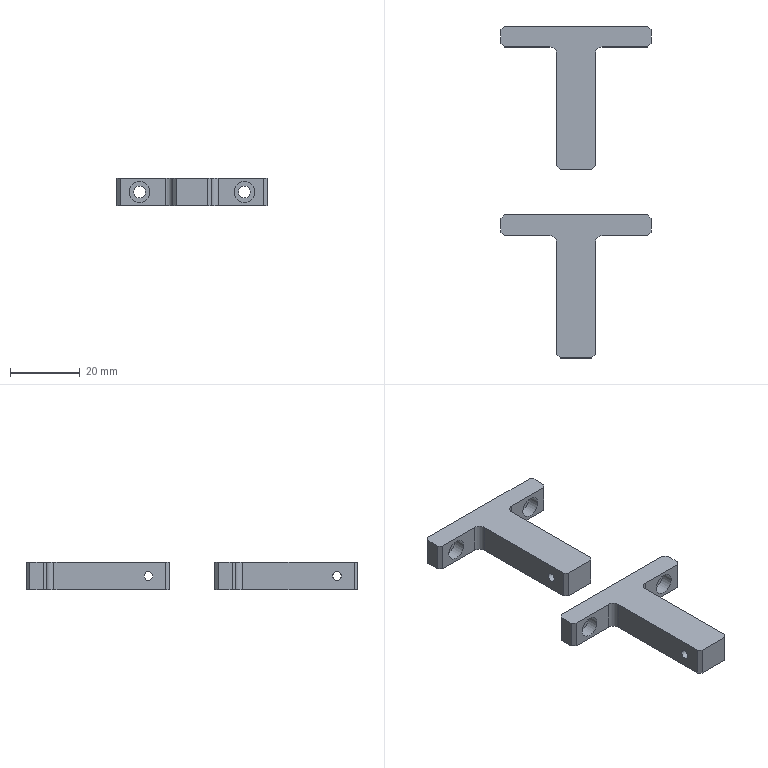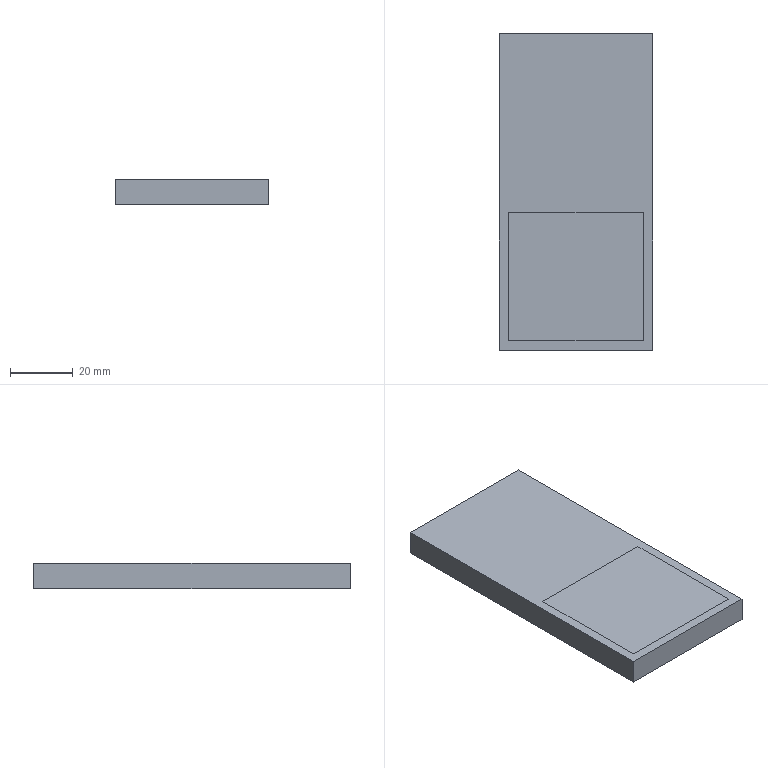CAM job | NX | 3+2 milling, drilling | part box 43 x 95 x 8 mm | stock box 49 x 101 x 8 mm
Tools:
number,name,description,diameter,corner_radius,flute_length,length,flutes
20,D10,Milling Tool-5 Parameters,10.0,0.0,50.0,75.0,2
15,D4,Milling Tool-5 Parameters,4.0,0.0,50.0,75.0,2
22,D6A45,Milling Tool-5 Parameters,6.0,0.0,3.0,3.0,2
3,3.4ZT,Drilling Tool,3.2,0.0,35.0,50.0,2
Operations:
program,operation,operation_type,tool,method,geometry_group,spindle_rpm,surface_speed,feed_per_tooth,feed_cut,feed_plunge,cut_length_mm,path_length_mm,cut_time_min,machine_time_min
1AB胶-100-50-8毛胚,ZLEVEL_PROFILE_COPY,ZLevelMilling,D10,METHOD,A,7500.0,235.0,0.1667,2500.0,100.0,4016.533,4231.633,1.607,1.628
1AB胶-100-50-8毛胚,ZLEVEL_PROFILE_COPY_COPY_2_1,ZLevelMilling,D4,METHOD,A,7501.0,94.0,0.0933,1400.0,100.0,629.154,1281.031,0.4494,0.5146
1AB胶-100-50-8毛胚,ZLEVEL_PROFILE_1_COPY_1_COPY_COPY,ZLevelMilling,D6A45,METHOD,A,7500.0,141.0,0.0667,1000.0,100.0,347.771,522.013,0.3478,0.3652
1AB胶-100-50-8毛胚,ZLEVEL_PROFILE_COPY_COPY_1,ZLevelMilling,D4,METHOD,A,7500.0,235.0,0.0667,1000.0,100.0,1132.708,1346.319,1.133,1.154
2,DRILLING_COPY_1_COPY_1,Operation,D6A45,METHOD,B,5000.0,94.0,0.025,250.0,0.0,8.0,179.15,0.032,0.0491
2,DRILLING_COPY_1_COPY_COPY_COPY_COPY_1_COPY_COPY_1_COPY_COPY_1_COPY,Operation,3.4ZT,METHOD,B,2000.0,20.0,0.0375,150.0,0.0,22.923,208.995,0.1528,0.1714
2,HOLE_MILLING_COPY_COPY_COPY,CylinderMilling,D4,METHOD,B,7500.0,70.0,0.0667,1000.0,100.0,264.018,559.818,0.264,0.2936